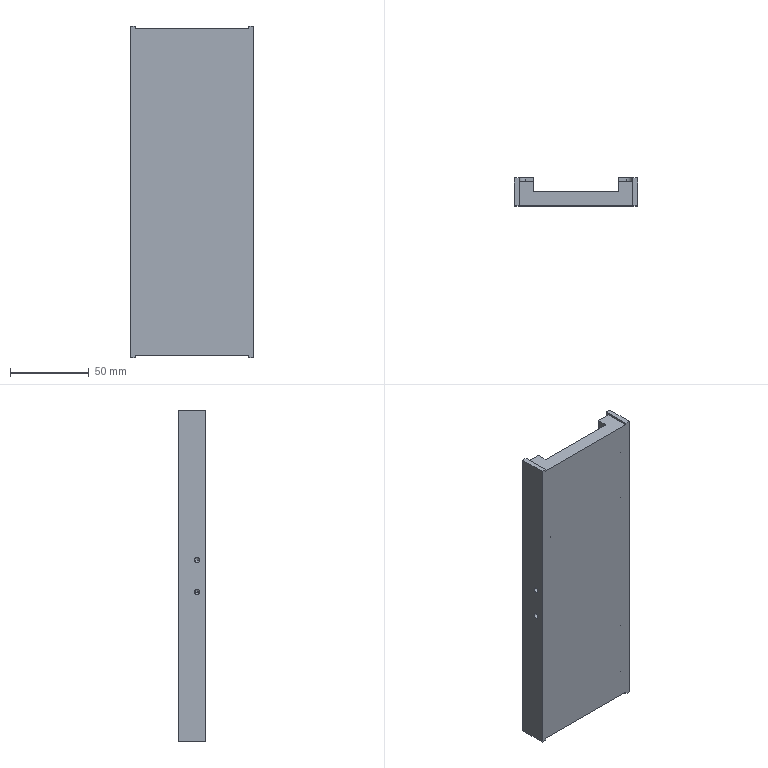Part | STEP file | FFH80-GY-004^FFH85-B3 -02_three-axis module | 1 solid | 88 faces | box 78 x 17.5 x 210 mm | volume 184560 mm3 | cylinder 34 | cone 28 | plane 26 | commonest cylinder face diameters 4.2 x16 3.3 x8 5 x4 8 x4 1 x2